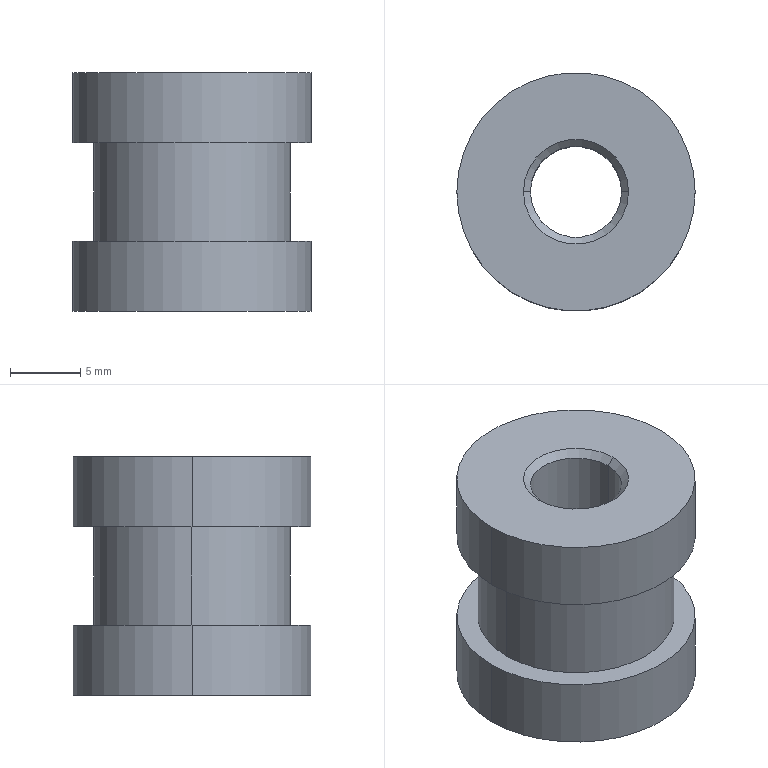Part | SolidWorks | features BaseBody 1 | 1 solid | 16 faces | box 17 x 17 x 17 mm | volume 2778 mm3 | cylinder 8 | cone 4 | plane 4 | commonest cylinder face diameters 17 x4 6.5 x2 14 x2
STEP:
#1=CARTESIAN_POINT('',(208.75,-197.,289.9));
#2=VERTEX_POINT('',#1);
#3=CARTESIAN_POINT('',(202.25,-197.,289.9));
#4=VERTEX_POINT('',#3);
#5=CARTESIAN_POINT('',(205.5,-197.,289.9));
#6=DIRECTION('',(0.,0.,-1.));
#7=DIRECTION('',(-1.,0.,0.));
#8=AXIS2_PLACEMENT_3D('',#5,#6,#7);
#9=CIRCLE('',#8,3.25);
#10=EDGE_CURVE('',#2,#4,#9,.T.);
#11=ORIENTED_EDGE('',*,*,#10,.T.);
#12=CARTESIAN_POINT('',(202.25,-197.,305.9));
#13=VERTEX_POINT('',#12);
#14=CARTESIAN_POINT('',(202.25,-197.,289.9));
#15=DIRECTION('',(0.,0.,1.));
#16=VECTOR('',#15,1000.);
#17=LINE('',#14,#16);
#18=EDGE_CURVE('',#4,#13,#17,.T.);
#19=ORIENTED_EDGE('',*,*,#18,.T.);
#20=CARTESIAN_POINT('',(208.75,-197.,305.9));
#21=VERTEX_POINT('',#20);
#22=CARTESIAN_POINT('',(205.5,-197.,305.9));
#23=DIRECTION('',(0.,0.,1.));
#24=DIRECTION('',(-1.,0.,0.));
#25=AXIS2_PLACEMENT_3D('',#22,#23,#24);
#26=CIRCLE('',#25,3.25);
#27=EDGE_CURVE('',#13,#21,#26,.T.);
#28=ORIENTED_EDGE('',*,*,#27,.T.);
#29=CARTESIAN_POINT('',(208.75,-197.,289.9));
#30=DIRECTION('',(0.,0.,1.));
#31=VECTOR('',#30,1000.);
#32=LINE('',#29,#31);
#33=EDGE_CURVE('',#2,#21,#32,.T.);
#34=ORIENTED_EDGE('',*,*,#33,.F.);
#35=EDGE_LOOP('',(#11,#19,#28,#34));
#36=FACE_OUTER_BOUND('',#35,.T.);
#37=CARTESIAN_POINT('',(205.5,-197.,289.9));
#38=DIRECTION('',(0.,0.,1.));
#39=DIRECTION('',(1.,0.,0.));
#40=AXIS2_PLACEMENT_3D('',#37,#38,#39);
#41=CYLINDRICAL_SURFACE('',#40,3.25);
#42=ADVANCED_FACE('',(#36),#41,.F.);
#43=CARTESIAN_POINT('',(205.5,-197.,289.9));
#44=DIRECTION('',(0.,0.,-1.));
#45=DIRECTION('',(-1.,0.,0.));
#46=AXIS2_PLACEMENT_3D('',#43,#44,#45);
#47=CIRCLE('',#46,3.25);
#48=EDGE_CURVE('',#4,#2,#47,.T.);
#49=ORIENTED_EDGE('',*,*,#48,.F.);
#50=CARTESIAN_POINT('',(201.75,-197.,289.4));
#51=VERTEX_POINT('',#50);
#52=CARTESIAN_POINT('',(204.5,-197.,292.15));
#53=DIRECTION('',(-0.7071,0.,-0.7071));
#54=VECTOR('',#53,1000.);
#55=LINE('',#52,#54);
#56=EDGE_CURVE('',#4,#51,#55,.T.);
#57=ORIENTED_EDGE('',*,*,#56,.T.);
#58=CARTESIAN_POINT('',(209.25,-197.,289.4));
#59=VERTEX_POINT('',#58);
#60=CARTESIAN_POINT('',(205.5,-197.,289.4));
#61=DIRECTION('',(0.,0.,1.));
#62=DIRECTION('',(-1.,0.,0.));
#63=AXIS2_PLACEMENT_3D('',#60,#61,#62);
#64=CIRCLE('',#63,3.75);
#65=EDGE_CURVE('',#59,#51,#64,.T.);
#66=ORIENTED_EDGE('',*,*,#65,.F.);
#67=CARTESIAN_POINT('',(206.5,-197.,292.15));
#68=DIRECTION('',(0.7071,0.,-0.7071));
#69=VECTOR('',#68,1000.);
#70=LINE('',#67,#69);
#71=EDGE_CURVE('',#2,#59,#70,.T.);
#72=ORIENTED_EDGE('',*,*,#71,.F.);
#73=EDGE_LOOP('',(#49,#57,#66,#72));
#74=FACE_OUTER_BOUND('',#73,.T.);
#75=CARTESIAN_POINT('',(205.5,-197.,292.15));
#76=DIRECTION('',(0.,0.,-1.));
#77=DIRECTION('',(1.,0.,0.));
#78=AXIS2_PLACEMENT_3D('',#75,#76,#77);
#79=CONICAL_SURFACE('',#78,1.,0.7854);
#80=ADVANCED_FACE('',(#74),#79,.F.);
#81=ORIENTED_EDGE('',*,*,#27,.F.);
#82=CARTESIAN_POINT('',(201.75,-197.,306.4));
#83=VERTEX_POINT('',#82);
#84=CARTESIAN_POINT('',(204.5,-197.,303.65));
#85=DIRECTION('',(-0.7071,0.,0.7071));
#86=VECTOR('',#85,1000.);
#87=LINE('',#84,#86);
#88=EDGE_CURVE('',#13,#83,#87,.T.);
#89=ORIENTED_EDGE('',*,*,#88,.T.);
#90=CARTESIAN_POINT('',(209.25,-197.,306.4));
#91=VERTEX_POINT('',#90);
#92=CARTESIAN_POINT('',(205.5,-197.,306.4));
#93=DIRECTION('',(0.,0.,-1.));
#94=DIRECTION('',(-1.,0.,0.));
#95=AXIS2_PLACEMENT_3D('',#92,#93,#94);
#96=CIRCLE('',#95,3.75);
#97=EDGE_CURVE('',#91,#83,#96,.T.);
#98=ORIENTED_EDGE('',*,*,#97,.F.);
#99=CARTESIAN_POINT('',(206.5,-197.,303.65));
#100=DIRECTION('',(0.7071,0.,0.7071));
#101=VECTOR('',#100,1000.);
#102=LINE('',#99,#101);
#103=EDGE_CURVE('',#21,#91,#102,.T.);
#104=ORIENTED_EDGE('',*,*,#103,.F.);
#105=EDGE_LOOP('',(#81,#89,#98,#104));
#106=FACE_OUTER_BOUND('',#105,.T.);
#107=CARTESIAN_POINT('',(205.5,-197.,303.65));
#108=DIRECTION('',(0.,0.,1.));
#109=DIRECTION('',(1.,0.,0.));
#110=AXIS2_PLACEMENT_3D('',#107,#108,#109);
#111=CONICAL_SURFACE('',#110,1.,0.7854);
#112=ADVANCED_FACE('',(#106),#111,.F.);
#113=CARTESIAN_POINT('',(197.,-197.,289.4));
#114=VERTEX_POINT('',#113);
#115=CARTESIAN_POINT('',(214.,-197.,289.4));
#116=VERTEX_POINT('',#115);
#117=CARTESIAN_POINT('',(205.5,-197.,289.4));
#118=DIRECTION('',(0.,0.,-1.));
#119=DIRECTION('',(-1.,0.,0.));
#120=AXIS2_PLACEMENT_3D('',#117,#118,#119);
#121=CIRCLE('',#120,8.5);
#122=EDGE_CURVE('',#114,#116,#121,.T.);
#123=ORIENTED_EDGE('',*,*,#122,.F.);
#124=CARTESIAN_POINT('',(197.,-197.,294.4));
#125=VERTEX_POINT('',#124);
#126=CARTESIAN_POINT('',(197.,-197.,289.4));
#127=DIRECTION('',(0.,0.,1.));
#128=VECTOR('',#127,1000.);
#129=LINE('',#126,#128);
#130=EDGE_CURVE('',#114,#125,#129,.T.);
#131=ORIENTED_EDGE('',*,*,#130,.T.);
#132=CARTESIAN_POINT('',(214.,-197.,294.4));
#133=VERTEX_POINT('',#132);
#134=CARTESIAN_POINT('',(205.5,-197.,294.4));
#135=DIRECTION('',(0.,0.,-1.));
#136=DIRECTION('',(-1.,0.,0.));
#137=AXIS2_PLACEMENT_3D('',#134,#135,#136);
#138=CIRCLE('',#137,8.5);
#139=EDGE_CURVE('',#125,#133,#138,.T.);
#140=ORIENTED_EDGE('',*,*,#139,.T.);
#141=CARTESIAN_POINT('',(214.,-197.,289.4));
#142=DIRECTION('',(0.,0.,1.));
#143=VECTOR('',#142,1000.);
#144=LINE('',#141,#143);
#145=EDGE_CURVE('',#116,#133,#144,.T.);
#146=ORIENTED_EDGE('',*,*,#145,.F.);
#147=EDGE_LOOP('',(#123,#131,#140,#146));
#148=FACE_OUTER_BOUND('',#147,.T.);
#149=CARTESIAN_POINT('',(205.5,-197.,289.4));
#150=DIRECTION('',(0.,0.,1.));
#151=DIRECTION('',(1.,0.,0.));
#152=AXIS2_PLACEMENT_3D('',#149,#150,#151);
#153=CYLINDRICAL_SURFACE('',#152,8.5);
#154=ADVANCED_FACE('',(#148),#153,.T.);
#155=CARTESIAN_POINT('',(214.,-197.,301.4));
#156=VERTEX_POINT('',#155);
#157=CARTESIAN_POINT('',(197.,-197.,301.4));
#158=VERTEX_POINT('',#157);
#159=CARTESIAN_POINT('',(205.5,-197.,301.4));
#160=DIRECTION('',(0.,0.,1.));
#161=DIRECTION('',(-1.,0.,0.));
#162=AXIS2_PLACEMENT_3D('',#159,#160,#161);
#163=CIRCLE('',#162,8.5);
#164=EDGE_CURVE('',#156,#158,#163,.T.);
#165=ORIENTED_EDGE('',*,*,#164,.T.);
#166=CARTESIAN_POINT('',(197.,-197.,306.4));
#167=VERTEX_POINT('',#166);
#168=CARTESIAN_POINT('',(197.,-197.,301.4));
#169=DIRECTION('',(0.,0.,1.));
#170=VECTOR('',#169,1000.);
#171=LINE('',#168,#170);
#172=EDGE_CURVE('',#158,#167,#171,.T.);
#173=ORIENTED_EDGE('',*,*,#172,.T.);
#174=CARTESIAN_POINT('',(214.,-197.,306.4));
#175=VERTEX_POINT('',#174);
#176=CARTESIAN_POINT('',(205.5,-197.,306.4));
#177=DIRECTION('',(0.,0.,1.));
#178=DIRECTION('',(-1.,0.,0.));
#179=AXIS2_PLACEMENT_3D('',#176,#177,#178);
#180=CIRCLE('',#179,8.5);
#181=EDGE_CURVE('',#175,#167,#180,.T.);
#182=ORIENTED_EDGE('',*,*,#181,.F.);
#183=CARTESIAN_POINT('',(214.,-197.,301.4));
#184=DIRECTION('',(0.,0.,1.));
#185=VECTOR('',#184,1000.);
#186=LINE('',#183,#185);
#187=EDGE_CURVE('',#156,#175,#186,.T.);
#188=ORIENTED_EDGE('',*,*,#187,.F.);
#189=EDGE_LOOP('',(#165,#173,#182,#188));
#190=FACE_OUTER_BOUND('',#189,.T.);
#191=CARTESIAN_POINT('',(205.5,-197.,301.4));
#192=DIRECTION('',(0.,0.,1.));
#193=DIRECTION('',(1.,0.,0.));
#194=AXIS2_PLACEMENT_3D('',#191,#192,#193);
#195=CYLINDRICAL_SURFACE('',#194,8.5);
#196=ADVANCED_FACE('',(#190),#195,.T.);
#197=CARTESIAN_POINT('',(212.5,-197.,301.4));
#198=VERTEX_POINT('',#197);
#199=CARTESIAN_POINT('',(198.5,-197.,301.4));
#200=VERTEX_POINT('',#199);
#201=CARTESIAN_POINT('',(205.5,-197.,301.4));
#202=DIRECTION('',(0.,0.,-1.));
#203=DIRECTION('',(-1.,0.,0.));
#204=AXIS2_PLACEMENT_3D('',#201,#202,#203);
#205=CIRCLE('',#204,7.);
#206=EDGE_CURVE('',#198,#200,#205,.T.);
#207=ORIENTED_EDGE('',*,*,#206,.T.);
#208=CARTESIAN_POINT('',(198.5,-197.,294.4));
#209=VERTEX_POINT('',#208);
#210=CARTESIAN_POINT('',(198.5,-197.,301.4));
#211=DIRECTION('',(0.,0.,-1.));
#212=VECTOR('',#211,1000.);
#213=LINE('',#210,#212);
#214=EDGE_CURVE('',#200,#209,#213,.T.);
#215=ORIENTED_EDGE('',*,*,#214,.T.);
#216=CARTESIAN_POINT('',(212.5,-197.,294.4));
#217=VERTEX_POINT('',#216);
#218=CARTESIAN_POINT('',(205.5,-197.,294.4));
#219=DIRECTION('',(0.,0.,-1.));
#220=DIRECTION('',(-1.,0.,0.));
#221=AXIS2_PLACEMENT_3D('',#218,#219,#220);
#222=CIRCLE('',#221,7.);
#223=EDGE_CURVE('',#217,#209,#222,.T.);
#224=ORIENTED_EDGE('',*,*,#223,.F.);
#225=CARTESIAN_POINT('',(212.5,-197.,301.4));
#226=DIRECTION('',(0.,0.,-1.));
#227=VECTOR('',#226,1000.);
#228=LINE('',#225,#227);
#229=EDGE_CURVE('',#198,#217,#228,.T.);
#230=ORIENTED_EDGE('',*,*,#229,.F.);
#231=EDGE_LOOP('',(#207,#215,#224,#230));
#232=FACE_OUTER_BOUND('',#231,.T.);
#233=CARTESIAN_POINT('',(205.5,-197.,301.4));
#234=DIRECTION('',(0.,0.,-1.));
#235=DIRECTION('',(1.,0.,0.));
#236=AXIS2_PLACEMENT_3D('',#233,#234,#235);
#237=CYLINDRICAL_SURFACE('',#236,7.);
#238=ADVANCED_FACE('',(#232),#237,.T.);
#239=ORIENTED_EDGE('',*,*,#206,.F.);
#240=CARTESIAN_POINT('',(205.5,-197.,301.4));
#241=DIRECTION('',(0.,0.,-1.));
#242=DIRECTION('',(-1.,0.,0.));
#243=AXIS2_PLACEMENT_3D('',#240,#241,#242);
#244=CIRCLE('',#243,7.);
#245=EDGE_CURVE('',#200,#198,#244,.T.);
#246=ORIENTED_EDGE('',*,*,#245,.F.);
#247=EDGE_LOOP('',(#239,#246));
#248=FACE_BOUND('',#247,.T.);
#249=ORIENTED_EDGE('',*,*,#164,.F.);
#250=CARTESIAN_POINT('',(205.5,-197.,301.4));
#251=DIRECTION('',(0.,0.,1.));
#252=DIRECTION('',(-1.,0.,0.));
#253=AXIS2_PLACEMENT_3D('',#250,#251,#252);
#254=CIRCLE('',#253,8.5);
#255=EDGE_CURVE('',#158,#156,#254,.T.);
#256=ORIENTED_EDGE('',*,*,#255,.F.);
#257=EDGE_LOOP('',(#249,#256));
#258=FACE_OUTER_BOUND('',#257,.T.);
#259=CARTESIAN_POINT('',(207.912,-197.,301.4));
#260=DIRECTION('',(0.,0.,-1.));
#261=DIRECTION('',(-1.,0.,0.));
#262=AXIS2_PLACEMENT_3D('',#259,#260,#261);
#263=PLANE('',#262);
#264=ADVANCED_FACE('',(#248,#258),#263,.T.);
#265=ORIENTED_EDGE('',*,*,#214,.F.);
#266=ORIENTED_EDGE('',*,*,#245,.T.);
#267=ORIENTED_EDGE('',*,*,#229,.T.);
#268=CARTESIAN_POINT('',(205.5,-197.,294.4));
#269=DIRECTION('',(0.,0.,-1.));
#270=DIRECTION('',(-1.,0.,0.));
#271=AXIS2_PLACEMENT_3D('',#268,#269,#270);
#272=CIRCLE('',#271,7.);
#273=EDGE_CURVE('',#209,#217,#272,.T.);
#274=ORIENTED_EDGE('',*,*,#273,.F.);
#275=EDGE_LOOP('',(#265,#266,#267,#274));
#276=FACE_OUTER_BOUND('',#275,.T.);
#277=CARTESIAN_POINT('',(205.5,-197.,301.4));
#278=DIRECTION('',(0.,0.,-1.));
#279=DIRECTION('',(1.,0.,0.));
#280=AXIS2_PLACEMENT_3D('',#277,#278,#279);
#281=CYLINDRICAL_SURFACE('',#280,7.);
#282=ADVANCED_FACE('',(#276),#281,.T.);
#283=ORIENTED_EDGE('',*,*,#223,.T.);
#284=ORIENTED_EDGE('',*,*,#273,.T.);
#285=EDGE_LOOP('',(#283,#284));
#286=FACE_BOUND('',#285,.T.);
#287=CARTESIAN_POINT('',(205.5,-197.,294.4));
#288=DIRECTION('',(0.,0.,-1.));
#289=DIRECTION('',(-1.,0.,0.));
#290=AXIS2_PLACEMENT_3D('',#287,#288,#289);
#291=CIRCLE('',#290,8.5);
#292=EDGE_CURVE('',#133,#125,#291,.T.);
#293=ORIENTED_EDGE('',*,*,#292,.F.);
#294=ORIENTED_EDGE('',*,*,#139,.F.);
#295=EDGE_LOOP('',(#293,#294));
#296=FACE_OUTER_BOUND('',#295,.T.);
#297=CARTESIAN_POINT('',(207.912,-197.,294.4));
#298=DIRECTION('',(0.,0.,1.));
#299=DIRECTION('',(0.,-1.,0.));
#300=AXIS2_PLACEMENT_3D('',#297,#298,#299);
#301=PLANE('',#300);
#302=ADVANCED_FACE('',(#286,#296),#301,.T.);
#303=ORIENTED_EDGE('',*,*,#172,.F.);
#304=ORIENTED_EDGE('',*,*,#255,.T.);
#305=ORIENTED_EDGE('',*,*,#187,.T.);
#306=CARTESIAN_POINT('',(205.5,-197.,306.4));
#307=DIRECTION('',(0.,0.,1.));
#308=DIRECTION('',(-1.,0.,0.));
#309=AXIS2_PLACEMENT_3D('',#306,#307,#308);
#310=CIRCLE('',#309,8.5);
#311=EDGE_CURVE('',#167,#175,#310,.T.);
#312=ORIENTED_EDGE('',*,*,#311,.F.);
#313=EDGE_LOOP('',(#303,#304,#305,#312));
#314=FACE_OUTER_BOUND('',#313,.T.);
#315=CARTESIAN_POINT('',(205.5,-197.,301.4));
#316=DIRECTION('',(0.,0.,1.));
#317=DIRECTION('',(1.,0.,0.));
#318=AXIS2_PLACEMENT_3D('',#315,#316,#317);
#319=CYLINDRICAL_SURFACE('',#318,8.5);
#320=ADVANCED_FACE('',(#314),#319,.T.);
#321=ORIENTED_EDGE('',*,*,#130,.F.);
#322=CARTESIAN_POINT('',(205.5,-197.,289.4));
#323=DIRECTION('',(0.,0.,-1.));
#324=DIRECTION('',(-1.,0.,0.));
#325=AXIS2_PLACEMENT_3D('',#322,#323,#324);
#326=CIRCLE('',#325,8.5);
#327=EDGE_CURVE('',#116,#114,#326,.T.);
#328=ORIENTED_EDGE('',*,*,#327,.F.);
#329=ORIENTED_EDGE('',*,*,#145,.T.);
#330=ORIENTED_EDGE('',*,*,#292,.T.);
#331=EDGE_LOOP('',(#321,#328,#329,#330));
#332=FACE_OUTER_BOUND('',#331,.T.);
#333=CARTESIAN_POINT('',(205.5,-197.,289.4));
#334=DIRECTION('',(0.,0.,1.));
#335=DIRECTION('',(1.,0.,0.));
#336=AXIS2_PLACEMENT_3D('',#333,#334,#335);
#337=CYLINDRICAL_SURFACE('',#336,8.5);
#338=ADVANCED_FACE('',(#332),#337,.T.);
#339=ORIENTED_EDGE('',*,*,#88,.F.);
#340=CARTESIAN_POINT('',(205.5,-197.,305.9));
#341=DIRECTION('',(0.,0.,1.));
#342=DIRECTION('',(-1.,0.,0.));
#343=AXIS2_PLACEMENT_3D('',#340,#341,#342);
#344=CIRCLE('',#343,3.25);
#345=EDGE_CURVE('',#21,#13,#344,.T.);
#346=ORIENTED_EDGE('',*,*,#345,.F.);
#347=ORIENTED_EDGE('',*,*,#103,.T.);
#348=CARTESIAN_POINT('',(205.5,-197.,306.4));
#349=DIRECTION('',(0.,0.,-1.));
#350=DIRECTION('',(-1.,0.,0.));
#351=AXIS2_PLACEMENT_3D('',#348,#349,#350);
#352=CIRCLE('',#351,3.75);
#353=EDGE_CURVE('',#83,#91,#352,.T.);
#354=ORIENTED_EDGE('',*,*,#353,.F.);
#355=EDGE_LOOP('',(#339,#346,#347,#354));
#356=FACE_OUTER_BOUND('',#355,.T.);
#357=CARTESIAN_POINT('',(205.5,-197.,303.65));
#358=DIRECTION('',(0.,0.,1.));
#359=DIRECTION('',(1.,0.,0.));
#360=AXIS2_PLACEMENT_3D('',#357,#358,#359);
#361=CONICAL_SURFACE('',#360,1.,0.7854);
#362=ADVANCED_FACE('',(#356),#361,.F.);
#363=ORIENTED_EDGE('',*,*,#56,.F.);
#364=ORIENTED_EDGE('',*,*,#10,.F.);
#365=ORIENTED_EDGE('',*,*,#71,.T.);
#366=CARTESIAN_POINT('',(205.5,-197.,289.4));
#367=DIRECTION('',(0.,0.,1.));
#368=DIRECTION('',(-1.,0.,0.));
#369=AXIS2_PLACEMENT_3D('',#366,#367,#368);
#370=CIRCLE('',#369,3.75);
#371=EDGE_CURVE('',#51,#59,#370,.T.);
#372=ORIENTED_EDGE('',*,*,#371,.F.);
#373=EDGE_LOOP('',(#363,#364,#365,#372));
#374=FACE_OUTER_BOUND('',#373,.T.);
#375=CARTESIAN_POINT('',(205.5,-197.,292.15));
#376=DIRECTION('',(0.,0.,-1.));
#377=DIRECTION('',(1.,0.,0.));
#378=AXIS2_PLACEMENT_3D('',#375,#376,#377);
#379=CONICAL_SURFACE('',#378,1.,0.7854);
#380=ADVANCED_FACE('',(#374),#379,.F.);
#381=ORIENTED_EDGE('',*,*,#18,.F.);
#382=ORIENTED_EDGE('',*,*,#48,.T.);
#383=ORIENTED_EDGE('',*,*,#33,.T.);
#384=ORIENTED_EDGE('',*,*,#345,.T.);
#385=EDGE_LOOP('',(#381,#382,#383,#384));
#386=FACE_OUTER_BOUND('',#385,.T.);
#387=CARTESIAN_POINT('',(205.5,-197.,289.9));
#388=DIRECTION('',(0.,0.,1.));
#389=DIRECTION('',(1.,0.,0.));
#390=AXIS2_PLACEMENT_3D('',#387,#388,#389);
#391=CYLINDRICAL_SURFACE('',#390,3.25);
#392=ADVANCED_FACE('',(#386),#391,.F.);
#393=ORIENTED_EDGE('',*,*,#97,.T.);
#394=ORIENTED_EDGE('',*,*,#353,.T.);
#395=EDGE_LOOP('',(#393,#394));
#396=FACE_BOUND('',#395,.T.);
#397=ORIENTED_EDGE('',*,*,#181,.T.);
#398=ORIENTED_EDGE('',*,*,#311,.T.);
#399=EDGE_LOOP('',(#397,#398));
#400=FACE_OUTER_BOUND('',#399,.T.);
#401=CARTESIAN_POINT('',(207.778,-197.,306.4));
#402=DIRECTION('',(0.,0.,1.));
#403=DIRECTION('',(0.,-1.,0.));
#404=AXIS2_PLACEMENT_3D('',#401,#402,#403);
#405=PLANE('',#404);
#406=ADVANCED_FACE('',(#396,#400),#405,.T.);
#407=ORIENTED_EDGE('',*,*,#65,.T.);
#408=ORIENTED_EDGE('',*,*,#371,.T.);
#409=EDGE_LOOP('',(#407,#408));
#410=FACE_BOUND('',#409,.T.);
#411=ORIENTED_EDGE('',*,*,#327,.T.);
#412=ORIENTED_EDGE('',*,*,#122,.T.);
#413=EDGE_LOOP('',(#411,#412));
#414=FACE_OUTER_BOUND('',#413,.T.);
#415=CARTESIAN_POINT('',(207.778,-197.,289.4));
#416=DIRECTION('',(0.,0.,-1.));
#417=DIRECTION('',(-1.,0.,0.));
#418=AXIS2_PLACEMENT_3D('',#415,#416,#417);
#419=PLANE('',#418);
#420=ADVANCED_FACE('',(#410,#414),#419,.T.);
#421=CLOSED_SHELL('',(#42,#80,#112,#154,#196,#238,#264,#282,#302,#320,#338,#362,#380,#392,#406,#420));
#422=MANIFOLD_SOLID_BREP('',#421);
#423=CARTESIAN_POINT('',(0.,0.,0.));
#424=DIRECTION('',(0.,0.,1.));
#425=DIRECTION('',(1.,0.,0.));
#426=AXIS2_PLACEMENT_3D('',#423,#424,#425);
#427=(LENGTH_UNIT()NAMED_UNIT(*)SI_UNIT(.MILLI.,.METRE.));
#428=UNCERTAINTY_MEASURE_WITH_UNIT(LENGTH_MEASURE(0.00001),#427,'','');
#429=(NAMED_UNIT(*)PLANE_ANGLE_UNIT()SI_UNIT($,.RADIAN.));
#430=(NAMED_UNIT(*)SI_UNIT($,.STERADIAN.)SOLID_ANGLE_UNIT());
#431=(GEOMETRIC_REPRESENTATION_CONTEXT(3)GLOBAL_UNCERTAINTY_ASSIGNED_CONTEXT((#428))GLOBAL_UNIT_ASSIGNED_CONTEXT((#427,#429,#430))REPRESENTATION_CONTEXT('',''));
#432=ADVANCED_BREP_SHAPE_REPRESENTATION('',(#422,#426),#431);